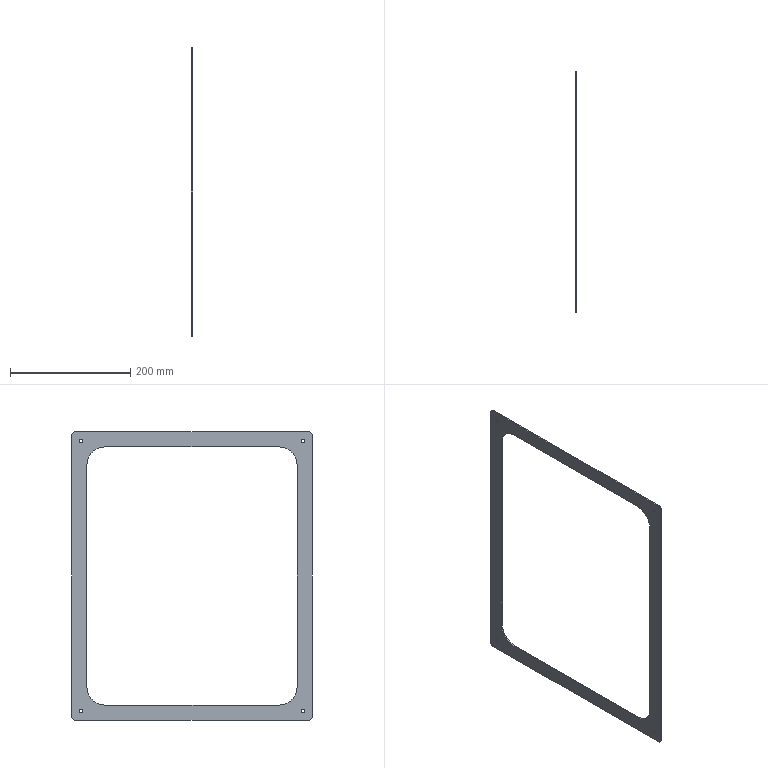Part | SolidWorks | features Fillet 2, ICE 2, Extrusion 1 | 1 solid | 26 faces | box 2 x 400 x 480 mm | volume 84276 mm3 | cylinder 16 | plane 10 | commonest cylinder face diameters 6 x8 10 x4 60 x4
STEP:
#1=CARTESIAN_POINT('',(0.,-185.,-222.));
#2=VERTEX_POINT('',#1);
#3=CARTESIAN_POINT('',(0.,-185.,-228.));
#4=VERTEX_POINT('',#3);
#5=CARTESIAN_POINT('',(0.,-185.,-225.));
#6=DIRECTION('',(1.,0.,0.));
#7=DIRECTION('',(0.,0.,-1.));
#8=AXIS2_PLACEMENT_3D('',#5,#6,#7);
#9=CIRCLE('',#8,3.);
#10=EDGE_CURVE('',#2,#4,#9,.T.);
#11=ORIENTED_EDGE('',*,*,#10,.F.);
#12=CARTESIAN_POINT('',(2.,-185.,-222.));
#13=VERTEX_POINT('',#12);
#14=CARTESIAN_POINT('',(0.,-185.,-222.));
#15=DIRECTION('',(1.,0.,0.));
#16=VECTOR('',#15,1000.);
#17=LINE('',#14,#16);
#18=EDGE_CURVE('',#2,#13,#17,.T.);
#19=ORIENTED_EDGE('',*,*,#18,.T.);
#20=CARTESIAN_POINT('',(2.,-185.,-228.));
#21=VERTEX_POINT('',#20);
#22=CARTESIAN_POINT('',(2.,-185.,-225.));
#23=DIRECTION('',(1.,0.,0.));
#24=DIRECTION('',(0.,0.,-1.));
#25=AXIS2_PLACEMENT_3D('',#22,#23,#24);
#26=CIRCLE('',#25,3.);
#27=EDGE_CURVE('',#13,#21,#26,.T.);
#28=ORIENTED_EDGE('',*,*,#27,.T.);
#29=CARTESIAN_POINT('',(0.,-185.,-228.));
#30=DIRECTION('',(1.,0.,0.));
#31=VECTOR('',#30,1000.);
#32=LINE('',#29,#31);
#33=EDGE_CURVE('',#4,#21,#32,.T.);
#34=ORIENTED_EDGE('',*,*,#33,.F.);
#35=EDGE_LOOP('',(#11,#19,#28,#34));
#36=FACE_OUTER_BOUND('',#35,.T.);
#37=CARTESIAN_POINT('',(0.,-185.,-225.));
#38=DIRECTION('',(1.,0.,0.));
#39=DIRECTION('',(0.,0.,-1.));
#40=AXIS2_PLACEMENT_3D('',#37,#38,#39);
#41=CYLINDRICAL_SURFACE('',#40,3.);
#42=ADVANCED_FACE('',(#36),#41,.F.);
#43=CARTESIAN_POINT('',(0.,-185.,228.));
#44=VERTEX_POINT('',#43);
#45=CARTESIAN_POINT('',(0.,-185.,222.));
#46=VERTEX_POINT('',#45);
#47=CARTESIAN_POINT('',(0.,-185.,225.));
#48=DIRECTION('',(1.,0.,0.));
#49=DIRECTION('',(0.,0.,-1.));
#50=AXIS2_PLACEMENT_3D('',#47,#48,#49);
#51=CIRCLE('',#50,3.);
#52=EDGE_CURVE('',#44,#46,#51,.T.);
#53=ORIENTED_EDGE('',*,*,#52,.F.);
#54=CARTESIAN_POINT('',(2.,-185.,228.));
#55=VERTEX_POINT('',#54);
#56=CARTESIAN_POINT('',(0.,-185.,228.));
#57=DIRECTION('',(1.,0.,0.));
#58=VECTOR('',#57,1000.);
#59=LINE('',#56,#58);
#60=EDGE_CURVE('',#44,#55,#59,.T.);
#61=ORIENTED_EDGE('',*,*,#60,.T.);
#62=CARTESIAN_POINT('',(2.,-185.,222.));
#63=VERTEX_POINT('',#62);
#64=CARTESIAN_POINT('',(2.,-185.,225.));
#65=DIRECTION('',(1.,0.,0.));
#66=DIRECTION('',(0.,0.,-1.));
#67=AXIS2_PLACEMENT_3D('',#64,#65,#66);
#68=CIRCLE('',#67,3.);
#69=EDGE_CURVE('',#55,#63,#68,.T.);
#70=ORIENTED_EDGE('',*,*,#69,.T.);
#71=CARTESIAN_POINT('',(0.,-185.,222.));
#72=DIRECTION('',(1.,0.,0.));
#73=VECTOR('',#72,1000.);
#74=LINE('',#71,#73);
#75=EDGE_CURVE('',#46,#63,#74,.T.);
#76=ORIENTED_EDGE('',*,*,#75,.F.);
#77=EDGE_LOOP('',(#53,#61,#70,#76));
#78=FACE_OUTER_BOUND('',#77,.T.);
#79=CARTESIAN_POINT('',(0.,-185.,225.));
#80=DIRECTION('',(1.,0.,0.));
#81=DIRECTION('',(0.,0.,-1.));
#82=AXIS2_PLACEMENT_3D('',#79,#80,#81);
#83=CYLINDRICAL_SURFACE('',#82,3.);
#84=ADVANCED_FACE('',(#78),#83,.F.);
#85=CARTESIAN_POINT('',(0.,185.,-222.));
#86=VERTEX_POINT('',#85);
#87=CARTESIAN_POINT('',(0.,185.,-228.));
#88=VERTEX_POINT('',#87);
#89=CARTESIAN_POINT('',(0.,185.,-225.));
#90=DIRECTION('',(1.,0.,0.));
#91=DIRECTION('',(0.,0.,-1.));
#92=AXIS2_PLACEMENT_3D('',#89,#90,#91);
#93=CIRCLE('',#92,3.);
#94=EDGE_CURVE('',#86,#88,#93,.T.);
#95=ORIENTED_EDGE('',*,*,#94,.F.);
#96=CARTESIAN_POINT('',(2.,185.,-222.));
#97=VERTEX_POINT('',#96);
#98=CARTESIAN_POINT('',(0.,185.,-222.));
#99=DIRECTION('',(1.,0.,0.));
#100=VECTOR('',#99,1000.);
#101=LINE('',#98,#100);
#102=EDGE_CURVE('',#86,#97,#101,.T.);
#103=ORIENTED_EDGE('',*,*,#102,.T.);
#104=CARTESIAN_POINT('',(2.,185.,-228.));
#105=VERTEX_POINT('',#104);
#106=CARTESIAN_POINT('',(2.,185.,-225.));
#107=DIRECTION('',(1.,0.,0.));
#108=DIRECTION('',(0.,0.,-1.));
#109=AXIS2_PLACEMENT_3D('',#106,#107,#108);
#110=CIRCLE('',#109,3.);
#111=EDGE_CURVE('',#97,#105,#110,.T.);
#112=ORIENTED_EDGE('',*,*,#111,.T.);
#113=CARTESIAN_POINT('',(0.,185.,-228.));
#114=DIRECTION('',(1.,0.,0.));
#115=VECTOR('',#114,1000.);
#116=LINE('',#113,#115);
#117=EDGE_CURVE('',#88,#105,#116,.T.);
#118=ORIENTED_EDGE('',*,*,#117,.F.);
#119=EDGE_LOOP('',(#95,#103,#112,#118));
#120=FACE_OUTER_BOUND('',#119,.T.);
#121=CARTESIAN_POINT('',(0.,185.,-225.));
#122=DIRECTION('',(1.,0.,0.));
#123=DIRECTION('',(0.,0.,-1.));
#124=AXIS2_PLACEMENT_3D('',#121,#122,#123);
#125=CYLINDRICAL_SURFACE('',#124,3.);
#126=ADVANCED_FACE('',(#120),#125,.F.);
#127=CARTESIAN_POINT('',(0.,185.,228.));
#128=VERTEX_POINT('',#127);
#129=CARTESIAN_POINT('',(0.,185.,222.));
#130=VERTEX_POINT('',#129);
#131=CARTESIAN_POINT('',(0.,185.,225.));
#132=DIRECTION('',(1.,0.,0.));
#133=DIRECTION('',(0.,0.,-1.));
#134=AXIS2_PLACEMENT_3D('',#131,#132,#133);
#135=CIRCLE('',#134,3.);
#136=EDGE_CURVE('',#128,#130,#135,.T.);
#137=ORIENTED_EDGE('',*,*,#136,.F.);
#138=CARTESIAN_POINT('',(2.,185.,228.));
#139=VERTEX_POINT('',#138);
#140=CARTESIAN_POINT('',(0.,185.,228.));
#141=DIRECTION('',(1.,0.,0.));
#142=VECTOR('',#141,1000.);
#143=LINE('',#140,#142);
#144=EDGE_CURVE('',#128,#139,#143,.T.);
#145=ORIENTED_EDGE('',*,*,#144,.T.);
#146=CARTESIAN_POINT('',(2.,185.,222.));
#147=VERTEX_POINT('',#146);
#148=CARTESIAN_POINT('',(2.,185.,225.));
#149=DIRECTION('',(1.,0.,0.));
#150=DIRECTION('',(0.,0.,-1.));
#151=AXIS2_PLACEMENT_3D('',#148,#149,#150);
#152=CIRCLE('',#151,3.);
#153=EDGE_CURVE('',#139,#147,#152,.T.);
#154=ORIENTED_EDGE('',*,*,#153,.T.);
#155=CARTESIAN_POINT('',(0.,185.,222.));
#156=DIRECTION('',(1.,0.,0.));
#157=VECTOR('',#156,1000.);
#158=LINE('',#155,#157);
#159=EDGE_CURVE('',#130,#147,#158,.T.);
#160=ORIENTED_EDGE('',*,*,#159,.F.);
#161=EDGE_LOOP('',(#137,#145,#154,#160));
#162=FACE_OUTER_BOUND('',#161,.T.);
#163=CARTESIAN_POINT('',(0.,185.,225.));
#164=DIRECTION('',(1.,0.,0.));
#165=DIRECTION('',(0.,0.,-1.));
#166=AXIS2_PLACEMENT_3D('',#163,#164,#165);
#167=CYLINDRICAL_SURFACE('',#166,3.);
#168=ADVANCED_FACE('',(#162),#167,.F.);
#169=CARTESIAN_POINT('',(0.,195.,240.));
#170=VERTEX_POINT('',#169);
#171=CARTESIAN_POINT('',(0.,-195.,240.));
#172=VERTEX_POINT('',#171);
#173=CARTESIAN_POINT('',(0.,200.,240.));
#174=DIRECTION('',(0.,-1.,0.));
#175=VECTOR('',#174,1000.);
#176=LINE('',#173,#175);
#177=EDGE_CURVE('',#170,#172,#176,.T.);
#178=ORIENTED_EDGE('',*,*,#177,.T.);
#179=CARTESIAN_POINT('',(2.,-195.,240.));
#180=VERTEX_POINT('',#179);
#181=CARTESIAN_POINT('',(2.,-195.,240.));
#182=DIRECTION('',(1.,0.,0.));
#183=VECTOR('',#182,1000.);
#184=LINE('',#181,#183);
#185=EDGE_CURVE('',#172,#180,#184,.T.);
#186=ORIENTED_EDGE('',*,*,#185,.T.);
#187=CARTESIAN_POINT('',(2.,195.,240.));
#188=VERTEX_POINT('',#187);
#189=CARTESIAN_POINT('',(2.,200.,240.));
#190=DIRECTION('',(0.,-1.,0.));
#191=VECTOR('',#190,1000.);
#192=LINE('',#189,#191);
#193=EDGE_CURVE('',#188,#180,#192,.T.);
#194=ORIENTED_EDGE('',*,*,#193,.F.);
#195=CARTESIAN_POINT('',(2.,195.,240.));
#196=DIRECTION('',(-1.,0.,0.));
#197=VECTOR('',#196,1000.);
#198=LINE('',#195,#197);
#199=EDGE_CURVE('',#188,#170,#198,.T.);
#200=ORIENTED_EDGE('',*,*,#199,.T.);
#201=EDGE_LOOP('',(#178,#186,#194,#200));
#202=FACE_OUTER_BOUND('',#201,.T.);
#203=CARTESIAN_POINT('',(2.,200.,240.));
#204=DIRECTION('',(0.,0.,-1.));
#205=DIRECTION('',(-1.,0.,0.));
#206=AXIS2_PLACEMENT_3D('',#203,#204,#205);
#207=PLANE('',#206);
#208=ADVANCED_FACE('',(#202),#207,.F.);
#209=CARTESIAN_POINT('',(2.,-200.,235.));
#210=VERTEX_POINT('',#209);
#211=CARTESIAN_POINT('',(2.,-200.,-235.));
#212=VERTEX_POINT('',#211);
#213=CARTESIAN_POINT('',(2.,-200.,240.));
#214=DIRECTION('',(0.,0.,-1.));
#215=VECTOR('',#214,1000.);
#216=LINE('',#213,#215);
#217=EDGE_CURVE('',#210,#212,#216,.T.);
#218=ORIENTED_EDGE('',*,*,#217,.F.);
#219=CARTESIAN_POINT('',(0.,-200.,235.));
#220=VERTEX_POINT('',#219);
#221=CARTESIAN_POINT('',(2.,-200.,235.));
#222=DIRECTION('',(-1.,0.,0.));
#223=VECTOR('',#222,1000.);
#224=LINE('',#221,#223);
#225=EDGE_CURVE('',#210,#220,#224,.T.);
#226=ORIENTED_EDGE('',*,*,#225,.T.);
#227=CARTESIAN_POINT('',(0.,-200.,-235.));
#228=VERTEX_POINT('',#227);
#229=CARTESIAN_POINT('',(0.,-200.,240.));
#230=DIRECTION('',(0.,0.,-1.));
#231=VECTOR('',#230,1000.);
#232=LINE('',#229,#231);
#233=EDGE_CURVE('',#220,#228,#232,.T.);
#234=ORIENTED_EDGE('',*,*,#233,.T.);
#235=CARTESIAN_POINT('',(2.,-200.,-235.));
#236=DIRECTION('',(1.,0.,0.));
#237=VECTOR('',#236,1000.);
#238=LINE('',#235,#237);
#239=EDGE_CURVE('',#228,#212,#238,.T.);
#240=ORIENTED_EDGE('',*,*,#239,.T.);
#241=EDGE_LOOP('',(#218,#226,#234,#240));
#242=FACE_OUTER_BOUND('',#241,.T.);
#243=CARTESIAN_POINT('',(2.,-200.,240.));
#244=DIRECTION('',(0.,1.,0.));
#245=DIRECTION('',(0.,0.,1.));
#246=AXIS2_PLACEMENT_3D('',#243,#244,#245);
#247=PLANE('',#246);
#248=ADVANCED_FACE('',(#242),#247,.F.);
#249=CARTESIAN_POINT('',(2.,-195.,-240.));
#250=VERTEX_POINT('',#249);
#251=CARTESIAN_POINT('',(2.,195.,-240.));
#252=VERTEX_POINT('',#251);
#253=CARTESIAN_POINT('',(2.,200.,-240.));
#254=DIRECTION('',(0.,1.,0.));
#255=VECTOR('',#254,1000.);
#256=LINE('',#253,#255);
#257=EDGE_CURVE('',#250,#252,#256,.T.);
#258=ORIENTED_EDGE('',*,*,#257,.F.);
#259=CARTESIAN_POINT('',(0.,-195.,-240.));
#260=VERTEX_POINT('',#259);
#261=CARTESIAN_POINT('',(2.,-195.,-240.));
#262=DIRECTION('',(-1.,0.,0.));
#263=VECTOR('',#262,1000.);
#264=LINE('',#261,#263);
#265=EDGE_CURVE('',#250,#260,#264,.T.);
#266=ORIENTED_EDGE('',*,*,#265,.T.);
#267=CARTESIAN_POINT('',(0.,195.,-240.));
#268=VERTEX_POINT('',#267);
#269=CARTESIAN_POINT('',(0.,200.,-240.));
#270=DIRECTION('',(0.,1.,0.));
#271=VECTOR('',#270,1000.);
#272=LINE('',#269,#271);
#273=EDGE_CURVE('',#260,#268,#272,.T.);
#274=ORIENTED_EDGE('',*,*,#273,.T.);
#275=CARTESIAN_POINT('',(2.,195.,-240.));
#276=DIRECTION('',(1.,0.,0.));
#277=VECTOR('',#276,1000.);
#278=LINE('',#275,#277);
#279=EDGE_CURVE('',#268,#252,#278,.T.);
#280=ORIENTED_EDGE('',*,*,#279,.T.);
#281=EDGE_LOOP('',(#258,#266,#274,#280));
#282=FACE_OUTER_BOUND('',#281,.T.);
#283=CARTESIAN_POINT('',(2.,200.,-240.));
#284=DIRECTION('',(0.,0.,1.));
#285=DIRECTION('',(1.,0.,0.));
#286=AXIS2_PLACEMENT_3D('',#283,#284,#285);
#287=PLANE('',#286);
#288=ADVANCED_FACE('',(#282),#287,.F.);
#289=CARTESIAN_POINT('',(2.,200.,-235.));
#290=VERTEX_POINT('',#289);
#291=CARTESIAN_POINT('',(2.,200.,235.));
#292=VERTEX_POINT('',#291);
#293=CARTESIAN_POINT('',(2.,200.,240.));
#294=DIRECTION('',(0.,0.,1.));
#295=VECTOR('',#294,1000.);
#296=LINE('',#293,#295);
#297=EDGE_CURVE('',#290,#292,#296,.T.);
#298=ORIENTED_EDGE('',*,*,#297,.F.);
#299=CARTESIAN_POINT('',(0.,200.,-235.));
#300=VERTEX_POINT('',#299);
#301=CARTESIAN_POINT('',(2.,200.,-235.));
#302=DIRECTION('',(-1.,0.,0.));
#303=VECTOR('',#302,1000.);
#304=LINE('',#301,#303);
#305=EDGE_CURVE('',#290,#300,#304,.T.);
#306=ORIENTED_EDGE('',*,*,#305,.T.);
#307=CARTESIAN_POINT('',(0.,200.,235.));
#308=VERTEX_POINT('',#307);
#309=CARTESIAN_POINT('',(0.,200.,240.));
#310=DIRECTION('',(0.,0.,1.));
#311=VECTOR('',#310,1000.);
#312=LINE('',#309,#311);
#313=EDGE_CURVE('',#300,#308,#312,.T.);
#314=ORIENTED_EDGE('',*,*,#313,.T.);
#315=CARTESIAN_POINT('',(2.,200.,235.));
#316=DIRECTION('',(1.,0.,0.));
#317=VECTOR('',#316,1000.);
#318=LINE('',#315,#317);
#319=EDGE_CURVE('',#308,#292,#318,.T.);
#320=ORIENTED_EDGE('',*,*,#319,.T.);
#321=EDGE_LOOP('',(#298,#306,#314,#320));
#322=FACE_OUTER_BOUND('',#321,.T.);
#323=CARTESIAN_POINT('',(2.,200.,240.));
#324=DIRECTION('',(0.,-1.,0.));
#325=DIRECTION('',(0.,0.,-1.));
#326=AXIS2_PLACEMENT_3D('',#323,#324,#325);
#327=PLANE('',#326);
#328=ADVANCED_FACE('',(#322),#327,.F.);
#329=CARTESIAN_POINT('',(2.,145.,215.));
#330=VERTEX_POINT('',#329);
#331=CARTESIAN_POINT('',(2.,-145.,215.));
#332=VERTEX_POINT('',#331);
#333=CARTESIAN_POINT('',(2.,175.,215.));
#334=DIRECTION('',(0.,-1.,0.));
#335=VECTOR('',#334,1000.);
#336=LINE('',#333,#335);
#337=EDGE_CURVE('',#330,#332,#336,.T.);
#338=ORIENTED_EDGE('',*,*,#337,.F.);
#339=CARTESIAN_POINT('',(2.,175.,185.));
#340=VERTEX_POINT('',#339);
#341=CARTESIAN_POINT('',(2.,145.,185.));
#342=DIRECTION('',(-1.,0.,0.));
#343=DIRECTION('',(0.,0.,-1.));
#344=AXIS2_PLACEMENT_3D('',#341,#342,#343);
#345=CIRCLE('',#344,30.);
#346=EDGE_CURVE('',#330,#340,#345,.T.);
#347=ORIENTED_EDGE('',*,*,#346,.T.);
#348=CARTESIAN_POINT('',(2.,175.,-185.));
#349=VERTEX_POINT('',#348);
#350=CARTESIAN_POINT('',(2.,175.,215.));
#351=DIRECTION('',(0.,0.,1.));
#352=VECTOR('',#351,1000.);
#353=LINE('',#350,#352);
#354=EDGE_CURVE('',#349,#340,#353,.T.);
#355=ORIENTED_EDGE('',*,*,#354,.F.);
#356=CARTESIAN_POINT('',(2.,145.,-215.));
#357=VERTEX_POINT('',#356);
#358=CARTESIAN_POINT('',(2.,145.,-185.));
#359=DIRECTION('',(-1.,0.,0.));
#360=DIRECTION('',(0.,0.,-1.));
#361=AXIS2_PLACEMENT_3D('',#358,#359,#360);
#362=CIRCLE('',#361,30.);
#363=EDGE_CURVE('',#349,#357,#362,.T.);
#364=ORIENTED_EDGE('',*,*,#363,.T.);
#365=CARTESIAN_POINT('',(2.,-145.,-215.));
#366=VERTEX_POINT('',#365);
#367=CARTESIAN_POINT('',(2.,175.,-215.));
#368=DIRECTION('',(0.,1.,0.));
#369=VECTOR('',#368,1000.);
#370=LINE('',#367,#369);
#371=EDGE_CURVE('',#366,#357,#370,.T.);
#372=ORIENTED_EDGE('',*,*,#371,.F.);
#373=CARTESIAN_POINT('',(2.,-175.,-185.));
#374=VERTEX_POINT('',#373);
#375=CARTESIAN_POINT('',(2.,-145.,-185.));
#376=DIRECTION('',(-1.,0.,0.));
#377=DIRECTION('',(0.,0.,-1.));
#378=AXIS2_PLACEMENT_3D('',#375,#376,#377);
#379=CIRCLE('',#378,30.);
#380=EDGE_CURVE('',#366,#374,#379,.T.);
#381=ORIENTED_EDGE('',*,*,#380,.T.);
#382=CARTESIAN_POINT('',(2.,-175.,185.));
#383=VERTEX_POINT('',#382);
#384=CARTESIAN_POINT('',(2.,-175.,215.));
#385=DIRECTION('',(0.,0.,-1.));
#386=VECTOR('',#385,1000.);
#387=LINE('',#384,#386);
#388=EDGE_CURVE('',#383,#374,#387,.T.);
#389=ORIENTED_EDGE('',*,*,#388,.F.);
#390=CARTESIAN_POINT('',(2.,-145.,185.));
#391=DIRECTION('',(-1.,0.,0.));
#392=DIRECTION('',(0.,0.,-1.));
#393=AXIS2_PLACEMENT_3D('',#390,#391,#392);
#394=CIRCLE('',#393,30.);
#395=EDGE_CURVE('',#383,#332,#394,.T.);
#396=ORIENTED_EDGE('',*,*,#395,.T.);
#397=EDGE_LOOP('',(#338,#347,#355,#364,#372,#381,#389,#396));
#398=FACE_BOUND('',#397,.T.);
#399=CARTESIAN_POINT('',(2.,-185.,-225.));
#400=DIRECTION('',(1.,0.,0.));
#401=DIRECTION('',(0.,0.,-1.));
#402=AXIS2_PLACEMENT_3D('',#399,#400,#401);
#403=CIRCLE('',#402,3.);
#404=EDGE_CURVE('',#21,#13,#403,.T.);
#405=ORIENTED_EDGE('',*,*,#404,.F.);
#406=ORIENTED_EDGE('',*,*,#27,.F.);
#407=EDGE_LOOP('',(#405,#406));
#408=FACE_BOUND('',#407,.T.);
#409=CARTESIAN_POINT('',(2.,-185.,225.));
#410=DIRECTION('',(1.,0.,0.));
#411=DIRECTION('',(0.,0.,-1.));
#412=AXIS2_PLACEMENT_3D('',#409,#410,#411);
#413=CIRCLE('',#412,3.);
#414=EDGE_CURVE('',#63,#55,#413,.T.);
#415=ORIENTED_EDGE('',*,*,#414,.F.);
#416=ORIENTED_EDGE('',*,*,#69,.F.);
#417=EDGE_LOOP('',(#415,#416));
#418=FACE_BOUND('',#417,.T.);
#419=CARTESIAN_POINT('',(2.,185.,-225.));
#420=DIRECTION('',(1.,0.,0.));
#421=DIRECTION('',(0.,0.,-1.));
#422=AXIS2_PLACEMENT_3D('',#419,#420,#421);
#423=CIRCLE('',#422,3.);
#424=EDGE_CURVE('',#105,#97,#423,.T.);
#425=ORIENTED_EDGE('',*,*,#424,.F.);
#426=ORIENTED_EDGE('',*,*,#111,.F.);
#427=EDGE_LOOP('',(#425,#426));
#428=FACE_BOUND('',#427,.T.);
#429=CARTESIAN_POINT('',(2.,185.,225.));
#430=DIRECTION('',(1.,0.,0.));
#431=DIRECTION('',(0.,0.,-1.));
#432=AXIS2_PLACEMENT_3D('',#429,#430,#431);
#433=CIRCLE('',#432,3.);
#434=EDGE_CURVE('',#147,#139,#433,.T.);
#435=ORIENTED_EDGE('',*,*,#434,.F.);
#436=ORIENTED_EDGE('',*,*,#153,.F.);
#437=EDGE_LOOP('',(#435,#436));
#438=FACE_BOUND('',#437,.T.);
#439=ORIENTED_EDGE('',*,*,#193,.T.);
#440=CARTESIAN_POINT('',(2.,-195.,235.));
#441=DIRECTION('',(1.,0.,0.));
#442=DIRECTION('',(0.,0.,-1.));
#443=AXIS2_PLACEMENT_3D('',#440,#441,#442);
#444=CIRCLE('',#443,5.);
#445=EDGE_CURVE('',#180,#210,#444,.T.);
#446=ORIENTED_EDGE('',*,*,#445,.T.);
#447=ORIENTED_EDGE('',*,*,#217,.T.);
#448=CARTESIAN_POINT('',(2.,-195.,-235.));
#449=DIRECTION('',(1.,0.,0.));
#450=DIRECTION('',(0.,0.,-1.));
#451=AXIS2_PLACEMENT_3D('',#448,#449,#450);
#452=CIRCLE('',#451,5.);
#453=EDGE_CURVE('',#212,#250,#452,.T.);
#454=ORIENTED_EDGE('',*,*,#453,.T.);
#455=ORIENTED_EDGE('',*,*,#257,.T.);
#456=CARTESIAN_POINT('',(2.,195.,-235.));
#457=DIRECTION('',(1.,0.,0.));
#458=DIRECTION('',(0.,0.,-1.));
#459=AXIS2_PLACEMENT_3D('',#456,#457,#458);
#460=CIRCLE('',#459,5.);
#461=EDGE_CURVE('',#252,#290,#460,.T.);
#462=ORIENTED_EDGE('',*,*,#461,.T.);
#463=ORIENTED_EDGE('',*,*,#297,.T.);
#464=CARTESIAN_POINT('',(2.,195.,235.));
#465=DIRECTION('',(1.,0.,0.));
#466=DIRECTION('',(0.,0.,-1.));
#467=AXIS2_PLACEMENT_3D('',#464,#465,#466);
#468=CIRCLE('',#467,5.);
#469=EDGE_CURVE('',#292,#188,#468,.T.);
#470=ORIENTED_EDGE('',*,*,#469,.T.);
#471=EDGE_LOOP('',(#439,#446,#447,#454,#455,#462,#463,#470));
#472=FACE_OUTER_BOUND('',#471,.T.);
#473=CARTESIAN_POINT('',(2.,0.,0.));
#474=DIRECTION('',(1.,0.,0.));
#475=DIRECTION('',(0.,0.,-1.));
#476=AXIS2_PLACEMENT_3D('',#473,#474,#475);
#477=PLANE('',#476);
#478=ADVANCED_FACE('',(#398,#408,#418,#428,#438,#472),#477,.T.);
#479=CARTESIAN_POINT('',(0.,-145.,-215.));
#480=VERTEX_POINT('',#479);
#481=CARTESIAN_POINT('',(0.,145.,-215.));
#482=VERTEX_POINT('',#481);
#483=CARTESIAN_POINT('',(0.,175.,-215.));
#484=DIRECTION('',(0.,1.,0.));
#485=VECTOR('',#484,1000.);
#486=LINE('',#483,#485);
#487=EDGE_CURVE('',#480,#482,#486,.T.);
#488=ORIENTED_EDGE('',*,*,#487,.T.);
#489=CARTESIAN_POINT('',(0.,175.,-185.));
#490=VERTEX_POINT('',#489);
#491=CARTESIAN_POINT('',(0.,145.,-185.));
#492=DIRECTION('',(1.,0.,0.));
#493=DIRECTION('',(0.,0.,-1.));
#494=AXIS2_PLACEMENT_3D('',#491,#492,#493);
#495=CIRCLE('',#494,30.);
#496=EDGE_CURVE('',#482,#490,#495,.T.);
#497=ORIENTED_EDGE('',*,*,#496,.T.);
#498=CARTESIAN_POINT('',(0.,175.,185.));
#499=VERTEX_POINT('',#498);
#500=CARTESIAN_POINT('',(0.,175.,215.));
#501=DIRECTION('',(0.,0.,1.));
#502=VECTOR('',#501,1000.);
#503=LINE('',#500,#502);
#504=EDGE_CURVE('',#490,#499,#503,.T.);
#505=ORIENTED_EDGE('',*,*,#504,.T.);
#506=CARTESIAN_POINT('',(0.,145.,215.));
#507=VERTEX_POINT('',#506);
#508=CARTESIAN_POINT('',(0.,145.,185.));
#509=DIRECTION('',(1.,0.,0.));
#510=DIRECTION('',(0.,0.,-1.));
#511=AXIS2_PLACEMENT_3D('',#508,#509,#510);
#512=CIRCLE('',#511,30.);
#513=EDGE_CURVE('',#499,#507,#512,.T.);
#514=ORIENTED_EDGE('',*,*,#513,.T.);
#515=CARTESIAN_POINT('',(0.,-145.,215.));
#516=VERTEX_POINT('',#515);
#517=CARTESIAN_POINT('',(0.,175.,215.));
#518=DIRECTION('',(0.,-1.,0.));
#519=VECTOR('',#518,1000.);
#520=LINE('',#517,#519);
#521=EDGE_CURVE('',#507,#516,#520,.T.);
#522=ORIENTED_EDGE('',*,*,#521,.T.);
#523=CARTESIAN_POINT('',(0.,-175.,185.));
#524=VERTEX_POINT('',#523);
#525=CARTESIAN_POINT('',(0.,-145.,185.));
#526=DIRECTION('',(1.,0.,0.));
#527=DIRECTION('',(0.,0.,-1.));
#528=AXIS2_PLACEMENT_3D('',#525,#526,#527);
#529=CIRCLE('',#528,30.);
#530=EDGE_CURVE('',#516,#524,#529,.T.);
#531=ORIENTED_EDGE('',*,*,#530,.T.);
#532=CARTESIAN_POINT('',(0.,-175.,-185.));
#533=VERTEX_POINT('',#532);
#534=CARTESIAN_POINT('',(0.,-175.,215.));
#535=DIRECTION('',(0.,0.,-1.));
#536=VECTOR('',#535,1000.);
#537=LINE('',#534,#536);
#538=EDGE_CURVE('',#524,#533,#537,.T.);
#539=ORIENTED_EDGE('',*,*,#538,.T.);
#540=CARTESIAN_POINT('',(0.,-145.,-185.));
#541=DIRECTION('',(1.,0.,0.));
#542=DIRECTION('',(0.,0.,-1.));
#543=AXIS2_PLACEMENT_3D('',#540,#541,#542);
#544=CIRCLE('',#543,30.);
#545=EDGE_CURVE('',#533,#480,#544,.T.);
#546=ORIENTED_EDGE('',*,*,#545,.T.);
#547=EDGE_LOOP('',(#488,#497,#505,#514,#522,#531,#539,#546));
#548=FACE_BOUND('',#547,.T.);
#549=CARTESIAN_POINT('',(0.,-185.,-225.));
#550=DIRECTION('',(1.,0.,0.));
#551=DIRECTION('',(0.,0.,-1.));
#552=AXIS2_PLACEMENT_3D('',#549,#550,#551);
#553=CIRCLE('',#552,3.);
#554=EDGE_CURVE('',#4,#2,#553,.T.);
#555=ORIENTED_EDGE('',*,*,#554,.T.);
#556=ORIENTED_EDGE('',*,*,#10,.T.);
#557=EDGE_LOOP('',(#555,#556));
#558=FACE_BOUND('',#557,.T.);
#559=CARTESIAN_POINT('',(0.,-185.,225.));
#560=DIRECTION('',(1.,0.,0.));
#561=DIRECTION('',(0.,0.,-1.));
#562=AXIS2_PLACEMENT_3D('',#559,#560,#561);
#563=CIRCLE('',#562,3.);
#564=EDGE_CURVE('',#46,#44,#563,.T.);
#565=ORIENTED_EDGE('',*,*,#564,.T.);
#566=ORIENTED_EDGE('',*,*,#52,.T.);
#567=EDGE_LOOP('',(#565,#566));
#568=FACE_BOUND('',#567,.T.);
#569=CARTESIAN_POINT('',(0.,185.,-225.));
#570=DIRECTION('',(1.,0.,0.));
#571=DIRECTION('',(0.,0.,-1.));
#572=AXIS2_PLACEMENT_3D('',#569,#570,#571);
#573=CIRCLE('',#572,3.);
#574=EDGE_CURVE('',#88,#86,#573,.T.);
#575=ORIENTED_EDGE('',*,*,#574,.T.);
#576=ORIENTED_EDGE('',*,*,#94,.T.);
#577=EDGE_LOOP('',(#575,#576));
#578=FACE_BOUND('',#577,.T.);
#579=CARTESIAN_POINT('',(0.,185.,225.));
#580=DIRECTION('',(1.,0.,0.));
#581=DIRECTION('',(0.,0.,-1.));
#582=AXIS2_PLACEMENT_3D('',#579,#580,#581);
#583=CIRCLE('',#582,3.);
#584=EDGE_CURVE('',#130,#128,#583,.T.);
#585=ORIENTED_EDGE('',*,*,#584,.T.);
#586=ORIENTED_EDGE('',*,*,#136,.T.);
#587=EDGE_LOOP('',(#585,#586));
#588=FACE_BOUND('',#587,.T.);
#589=ORIENTED_EDGE('',*,*,#233,.F.);
#590=CARTESIAN_POINT('',(0.,-195.,235.));
#591=DIRECTION('',(-1.,0.,0.));
#592=DIRECTION('',(0.,0.,-1.));
#593=AXIS2_PLACEMENT_3D('',#590,#591,#592);
#594=CIRCLE('',#593,5.);
#595=EDGE_CURVE('',#220,#172,#594,.T.);
#596=ORIENTED_EDGE('',*,*,#595,.T.);
#597=ORIENTED_EDGE('',*,*,#177,.F.);
#598=CARTESIAN_POINT('',(0.,195.,235.));
#599=DIRECTION('',(-1.,0.,0.));
#600=DIRECTION('',(0.,0.,-1.));
#601=AXIS2_PLACEMENT_3D('',#598,#599,#600);
#602=CIRCLE('',#601,5.);
#603=EDGE_CURVE('',#170,#308,#602,.T.);
#604=ORIENTED_EDGE('',*,*,#603,.T.);
#605=ORIENTED_EDGE('',*,*,#313,.F.);
#606=CARTESIAN_POINT('',(0.,195.,-235.));
#607=DIRECTION('',(-1.,0.,0.));
#608=DIRECTION('',(0.,0.,-1.));
#609=AXIS2_PLACEMENT_3D('',#606,#607,#608);
#610=CIRCLE('',#609,5.);
#611=EDGE_CURVE('',#300,#268,#610,.T.);
#612=ORIENTED_EDGE('',*,*,#611,.T.);
#613=ORIENTED_EDGE('',*,*,#273,.F.);
#614=CARTESIAN_POINT('',(0.,-195.,-235.));
#615=DIRECTION('',(-1.,0.,0.));
#616=DIRECTION('',(0.,0.,-1.));
#617=AXIS2_PLACEMENT_3D('',#614,#615,#616);
#618=CIRCLE('',#617,5.);
#619=EDGE_CURVE('',#260,#228,#618,.T.);
#620=ORIENTED_EDGE('',*,*,#619,.T.);
#621=EDGE_LOOP('',(#589,#596,#597,#604,#605,#612,#613,#620));
#622=FACE_OUTER_BOUND('',#621,.T.);
#623=CARTESIAN_POINT('',(0.,0.,0.));
#624=DIRECTION('',(1.,0.,0.));
#625=DIRECTION('',(0.,0.,-1.));
#626=AXIS2_PLACEMENT_3D('',#623,#624,#625);
#627=PLANE('',#626);
#628=ADVANCED_FACE('',(#548,#558,#568,#578,#588,#622),#627,.F.);
#629=ORIENTED_EDGE('',*,*,#144,.F.);
#630=ORIENTED_EDGE('',*,*,#584,.F.);
#631=ORIENTED_EDGE('',*,*,#159,.T.);
#632=ORIENTED_EDGE('',*,*,#434,.T.);
#633=EDGE_LOOP('',(#629,#630,#631,#632));
#634=FACE_OUTER_BOUND('',#633,.T.);
#635=CARTESIAN_POINT('',(0.,185.,225.));
#636=DIRECTION('',(1.,0.,0.));
#637=DIRECTION('',(0.,0.,-1.));
#638=AXIS2_PLACEMENT_3D('',#635,#636,#637);
#639=CYLINDRICAL_SURFACE('',#638,3.);
#640=ADVANCED_FACE('',(#634),#639,.F.);
#641=ORIENTED_EDGE('',*,*,#102,.F.);
#642=ORIENTED_EDGE('',*,*,#574,.F.);
#643=ORIENTED_EDGE('',*,*,#117,.T.);
#644=ORIENTED_EDGE('',*,*,#424,.T.);
#645=EDGE_LOOP('',(#641,#642,#643,#644));
#646=FACE_OUTER_BOUND('',#645,.T.);
#647=CARTESIAN_POINT('',(0.,185.,-225.));
#648=DIRECTION('',(1.,0.,0.));
#649=DIRECTION('',(0.,0.,-1.));
#650=AXIS2_PLACEMENT_3D('',#647,#648,#649);
#651=CYLINDRICAL_SURFACE('',#650,3.);
#652=ADVANCED_FACE('',(#646),#651,.F.);
#653=ORIENTED_EDGE('',*,*,#60,.F.);
#654=ORIENTED_EDGE('',*,*,#564,.F.);
#655=ORIENTED_EDGE('',*,*,#75,.T.);
#656=ORIENTED_EDGE('',*,*,#414,.T.);
#657=EDGE_LOOP('',(#653,#654,#655,#656));
#658=FACE_OUTER_BOUND('',#657,.T.);
#659=CARTESIAN_POINT('',(0.,-185.,225.));
#660=DIRECTION('',(1.,0.,0.));
#661=DIRECTION('',(0.,0.,-1.));
#662=AXIS2_PLACEMENT_3D('',#659,#660,#661);
#663=CYLINDRICAL_SURFACE('',#662,3.);
#664=ADVANCED_FACE('',(#658),#663,.F.);
#665=ORIENTED_EDGE('',*,*,#18,.F.);
#666=ORIENTED_EDGE('',*,*,#554,.F.);
#667=ORIENTED_EDGE('',*,*,#33,.T.);
#668=ORIENTED_EDGE('',*,*,#404,.T.);
#669=EDGE_LOOP('',(#665,#666,#667,#668));
#670=FACE_OUTER_BOUND('',#669,.T.);
#671=CARTESIAN_POINT('',(0.,-185.,-225.));
#672=DIRECTION('',(1.,0.,0.));
#673=DIRECTION('',(0.,0.,-1.));
#674=AXIS2_PLACEMENT_3D('',#671,#672,#673);
#675=CYLINDRICAL_SURFACE('',#674,3.);
#676=ADVANCED_FACE('',(#670),#675,.F.);
#677=ORIENTED_EDGE('',*,*,#445,.F.);
#678=ORIENTED_EDGE('',*,*,#185,.F.);
#679=ORIENTED_EDGE('',*,*,#595,.F.);
#680=ORIENTED_EDGE('',*,*,#225,.F.);
#681=EDGE_LOOP('',(#677,#678,#679,#680));
#682=FACE_OUTER_BOUND('',#681,.T.);
#683=CARTESIAN_POINT('',(2.,-195.,235.));
#684=DIRECTION('',(-1.,0.,0.));
#685=DIRECTION('',(0.,0.,1.));
#686=AXIS2_PLACEMENT_3D('',#683,#684,#685);
#687=CYLINDRICAL_SURFACE('',#686,5.);
#688=ADVANCED_FACE('',(#682),#687,.T.);
#689=ORIENTED_EDGE('',*,*,#453,.F.);
#690=ORIENTED_EDGE('',*,*,#239,.F.);
#691=ORIENTED_EDGE('',*,*,#619,.F.);
#692=ORIENTED_EDGE('',*,*,#265,.F.);
#693=EDGE_LOOP('',(#689,#690,#691,#692));
#694=FACE_OUTER_BOUND('',#693,.T.);
#695=CARTESIAN_POINT('',(2.,-195.,-235.));
#696=DIRECTION('',(-1.,0.,0.));
#697=DIRECTION('',(0.,0.,1.));
#698=AXIS2_PLACEMENT_3D('',#695,#696,#697);
#699=CYLINDRICAL_SURFACE('',#698,5.);
#700=ADVANCED_FACE('',(#694),#699,.T.);
#701=ORIENTED_EDGE('',*,*,#461,.F.);
#702=ORIENTED_EDGE('',*,*,#279,.F.);
#703=ORIENTED_EDGE('',*,*,#611,.F.);
#704=ORIENTED_EDGE('',*,*,#305,.F.);
#705=EDGE_LOOP('',(#701,#702,#703,#704));
#706=FACE_OUTER_BOUND('',#705,.T.);
#707=CARTESIAN_POINT('',(2.,195.,-235.));
#708=DIRECTION('',(-1.,0.,0.));
#709=DIRECTION('',(0.,0.,1.));
#710=AXIS2_PLACEMENT_3D('',#707,#708,#709);
#711=CYLINDRICAL_SURFACE('',#710,5.);
#712=ADVANCED_FACE('',(#706),#711,.T.);
#713=ORIENTED_EDGE('',*,*,#469,.F.);
#714=ORIENTED_EDGE('',*,*,#319,.F.);
#715=ORIENTED_EDGE('',*,*,#603,.F.);
#716=ORIENTED_EDGE('',*,*,#199,.F.);
#717=EDGE_LOOP('',(#713,#714,#715,#716));
#718=FACE_OUTER_BOUND('',#717,.T.);
#719=CARTESIAN_POINT('',(2.,195.,235.));
#720=DIRECTION('',(-1.,0.,0.));
#721=DIRECTION('',(0.,0.,1.));
#722=AXIS2_PLACEMENT_3D('',#719,#720,#721);
#723=CYLINDRICAL_SURFACE('',#722,5.);
#724=ADVANCED_FACE('',(#718),#723,.T.);
#725=ORIENTED_EDGE('',*,*,#337,.T.);
#726=CARTESIAN_POINT('',(0.,-145.,215.));
#727=DIRECTION('',(-1.,0.,0.));
#728=VECTOR('',#727,1000.);
#729=LINE('',#726,#728);
#730=EDGE_CURVE('',#332,#516,#729,.T.);
#731=ORIENTED_EDGE('',*,*,#730,.T.);
#732=ORIENTED_EDGE('',*,*,#521,.F.);
#733=CARTESIAN_POINT('',(2.,145.,215.));
#734=DIRECTION('',(1.,0.,0.));
#735=VECTOR('',#734,1000.);
#736=LINE('',#733,#735);
#737=EDGE_CURVE('',#507,#330,#736,.T.);
#738=ORIENTED_EDGE('',*,*,#737,.T.);
#739=EDGE_LOOP('',(#725,#731,#732,#738));
#740=FACE_OUTER_BOUND('',#739,.T.);
#741=CARTESIAN_POINT('',(0.,175.,215.));
#742=DIRECTION('',(0.,0.,1.));
#743=DIRECTION('',(0.,-1.,0.));
#744=AXIS2_PLACEMENT_3D('',#741,#742,#743);
#745=PLANE('',#744);
#746=ADVANCED_FACE('',(#740),#745,.F.);
#747=ORIENTED_EDGE('',*,*,#504,.F.);
#748=CARTESIAN_POINT('',(2.,175.,-185.));
#749=DIRECTION('',(1.,0.,0.));
#750=VECTOR('',#749,1000.);
#751=LINE('',#748,#750);
#752=EDGE_CURVE('',#490,#349,#751,.T.);
#753=ORIENTED_EDGE('',*,*,#752,.T.);
#754=ORIENTED_EDGE('',*,*,#354,.T.);
#755=CARTESIAN_POINT('',(0.,175.,185.));
#756=DIRECTION('',(-1.,0.,0.));
#757=VECTOR('',#756,1000.);
#758=LINE('',#755,#757);
#759=EDGE_CURVE('',#340,#499,#758,.T.);
#760=ORIENTED_EDGE('',*,*,#759,.T.);
#761=EDGE_LOOP('',(#747,#753,#754,#760));
#762=FACE_OUTER_BOUND('',#761,.T.);
#763=CARTESIAN_POINT('',(0.,175.,215.));
#764=DIRECTION('',(0.,1.,0.));
#765=DIRECTION('',(0.,0.,1.));
#766=AXIS2_PLACEMENT_3D('',#763,#764,#765);
#767=PLANE('',#766);
#768=ADVANCED_FACE('',(#762),#767,.F.);
#769=ORIENTED_EDGE('',*,*,#487,.F.);
#770=CARTESIAN_POINT('',(2.,-145.,-215.));
#771=DIRECTION('',(1.,0.,0.));
#772=VECTOR('',#771,1000.);
#773=LINE('',#770,#772);
#774=EDGE_CURVE('',#480,#366,#773,.T.);
#775=ORIENTED_EDGE('',*,*,#774,.T.);
#776=ORIENTED_EDGE('',*,*,#371,.T.);
#777=CARTESIAN_POINT('',(0.,145.,-215.));
#778=DIRECTION('',(-1.,0.,0.));
#779=VECTOR('',#778,1000.);
#780=LINE('',#777,#779);
#781=EDGE_CURVE('',#357,#482,#780,.T.);
#782=ORIENTED_EDGE('',*,*,#781,.T.);
#783=EDGE_LOOP('',(#769,#775,#776,#782));
#784=FACE_OUTER_BOUND('',#783,.T.);
#785=CARTESIAN_POINT('',(0.,175.,-215.));
#786=DIRECTION('',(0.,0.,-1.));
#787=DIRECTION('',(0.,1.,0.));
#788=AXIS2_PLACEMENT_3D('',#785,#786,#787);
#789=PLANE('',#788);
#790=ADVANCED_FACE('',(#784),#789,.F.);
#791=ORIENTED_EDGE('',*,*,#538,.F.);
#792=CARTESIAN_POINT('',(2.,-175.,185.));
#793=DIRECTION('',(1.,0.,0.));
#794=VECTOR('',#793,1000.);
#795=LINE('',#792,#794);
#796=EDGE_CURVE('',#524,#383,#795,.T.);
#797=ORIENTED_EDGE('',*,*,#796,.T.);
#798=ORIENTED_EDGE('',*,*,#388,.T.);
#799=CARTESIAN_POINT('',(0.,-175.,-185.));
#800=DIRECTION('',(-1.,0.,0.));
#801=VECTOR('',#800,1000.);
#802=LINE('',#799,#801);
#803=EDGE_CURVE('',#374,#533,#802,.T.);
#804=ORIENTED_EDGE('',*,*,#803,.T.);
#805=EDGE_LOOP('',(#791,#797,#798,#804));
#806=FACE_OUTER_BOUND('',#805,.T.);
#807=CARTESIAN_POINT('',(0.,-175.,215.));
#808=DIRECTION('',(0.,-1.,0.));
#809=DIRECTION('',(0.,0.,-1.));
#810=AXIS2_PLACEMENT_3D('',#807,#808,#809);
#811=PLANE('',#810);
#812=ADVANCED_FACE('',(#806),#811,.F.);
#813=ORIENTED_EDGE('',*,*,#530,.F.);
#814=ORIENTED_EDGE('',*,*,#730,.F.);
#815=ORIENTED_EDGE('',*,*,#395,.F.);
#816=ORIENTED_EDGE('',*,*,#796,.F.);
#817=EDGE_LOOP('',(#813,#814,#815,#816));
#818=FACE_OUTER_BOUND('',#817,.T.);
#819=CARTESIAN_POINT('',(0.,-145.,185.));
#820=DIRECTION('',(-1.,0.,0.));
#821=DIRECTION('',(0.,0.,1.));
#822=AXIS2_PLACEMENT_3D('',#819,#820,#821);
#823=CYLINDRICAL_SURFACE('',#822,30.);
#824=ADVANCED_FACE('',(#818),#823,.F.);
#825=ORIENTED_EDGE('',*,*,#545,.F.);
#826=ORIENTED_EDGE('',*,*,#803,.F.);
#827=ORIENTED_EDGE('',*,*,#380,.F.);
#828=ORIENTED_EDGE('',*,*,#774,.F.);
#829=EDGE_LOOP('',(#825,#826,#827,#828));
#830=FACE_OUTER_BOUND('',#829,.T.);
#831=CARTESIAN_POINT('',(0.,-145.,-185.));
#832=DIRECTION('',(-1.,0.,0.));
#833=DIRECTION('',(0.,0.,1.));
#834=AXIS2_PLACEMENT_3D('',#831,#832,#833);
#835=CYLINDRICAL_SURFACE('',#834,30.);
#836=ADVANCED_FACE('',(#830),#835,.F.);
#837=ORIENTED_EDGE('',*,*,#496,.F.);
#838=ORIENTED_EDGE('',*,*,#781,.F.);
#839=ORIENTED_EDGE('',*,*,#363,.F.);
#840=ORIENTED_EDGE('',*,*,#752,.F.);
#841=EDGE_LOOP('',(#837,#838,#839,#840));
#842=FACE_OUTER_BOUND('',#841,.T.);
#843=CARTESIAN_POINT('',(0.,145.,-185.));
#844=DIRECTION('',(-1.,0.,0.));
#845=DIRECTION('',(0.,0.,1.));
#846=AXIS2_PLACEMENT_3D('',#843,#844,#845);
#847=CYLINDRICAL_SURFACE('',#846,30.);
#848=ADVANCED_FACE('',(#842),#847,.F.);
#849=ORIENTED_EDGE('',*,*,#513,.F.);
#850=ORIENTED_EDGE('',*,*,#759,.F.);
#851=ORIENTED_EDGE('',*,*,#346,.F.);
#852=ORIENTED_EDGE('',*,*,#737,.F.);
#853=EDGE_LOOP('',(#849,#850,#851,#852));
#854=FACE_OUTER_BOUND('',#853,.T.);
#855=CARTESIAN_POINT('',(0.,145.,185.));
#856=DIRECTION('',(-1.,0.,0.));
#857=DIRECTION('',(0.,0.,1.));
#858=AXIS2_PLACEMENT_3D('',#855,#856,#857);
#859=CYLINDRICAL_SURFACE('',#858,30.);
#860=ADVANCED_FACE('',(#854),#859,.F.);
#861=CLOSED_SHELL('',(#42,#84,#126,#168,#208,#248,#288,#328,#478,#628,#640,#652,#664,#676,#688,#700,#712,#724,#746,#768,#790,#812,#824,#836,#848,#860));
#862=MANIFOLD_SOLID_BREP('',#861);
#863=CARTESIAN_POINT('',(0.,0.,0.));
#864=DIRECTION('',(0.,0.,1.));
#865=DIRECTION('',(1.,0.,0.));
#866=AXIS2_PLACEMENT_3D('',#863,#864,#865);
#867=(LENGTH_UNIT()NAMED_UNIT(*)SI_UNIT(.MILLI.,.METRE.));
#868=UNCERTAINTY_MEASURE_WITH_UNIT(LENGTH_MEASURE(0.00001),#867,'','');
#869=(NAMED_UNIT(*)PLANE_ANGLE_UNIT()SI_UNIT($,.RADIAN.));
#870=(NAMED_UNIT(*)SI_UNIT($,.STERADIAN.)SOLID_ANGLE_UNIT());
#871=(GEOMETRIC_REPRESENTATION_CONTEXT(3)GLOBAL_UNCERTAINTY_ASSIGNED_CONTEXT((#868))GLOBAL_UNIT_ASSIGNED_CONTEXT((#867,#869,#870))REPRESENTATION_CONTEXT('',''));
#872=ADVANCED_BREP_SHAPE_REPRESENTATION('',(#862,#866),#871);